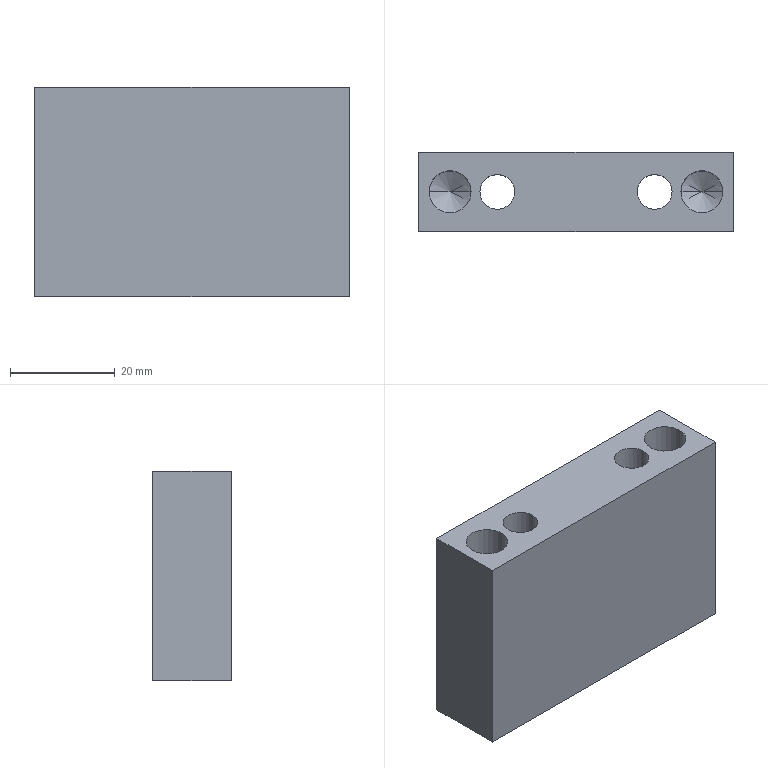Part | STEP file | 11-FG-SJ00611 | 1 solid | 24 faces | box 60 x 15 x 40 mm | volume 29373 mm3 | cylinder 12 | plane 8 | cone 4 | commonest cylinder face diameters 6.6 x4 8 x4 11 x4
STEP:
#1=CARTESIAN_POINT('',(-28.,0.,28.));
#2=VERTEX_POINT('',#1);
#3=CARTESIAN_POINT('',(-20.,0.,28.));
#4=VERTEX_POINT('',#3);
#5=CARTESIAN_POINT('',(-24.,0.,28.));
#6=DIRECTION('',(0.,0.,1.));
#7=DIRECTION('',(1.,0.,0.));
#8=AXIS2_PLACEMENT_3D('',#5,#6,#7);
#9=CIRCLE('',#8,4.);
#10=EDGE_CURVE('',#2,#4,#9,.T.);
#11=ORIENTED_EDGE('',*,*,#10,.F.);
#12=CARTESIAN_POINT('',(-28.,0.,40.));
#13=VERTEX_POINT('',#12);
#14=CARTESIAN_POINT('',(-28.,0.,40.));
#15=DIRECTION('',(0.,0.,1.));
#16=VECTOR('',#15,1000.);
#17=LINE('',#14,#16);
#18=EDGE_CURVE('',#2,#13,#17,.T.);
#19=ORIENTED_EDGE('',*,*,#18,.T.);
#20=CARTESIAN_POINT('',(-20.,0.,40.));
#21=VERTEX_POINT('',#20);
#22=CARTESIAN_POINT('',(-24.,0.,40.));
#23=DIRECTION('',(0.,0.,1.));
#24=DIRECTION('',(1.,0.,0.));
#25=AXIS2_PLACEMENT_3D('',#22,#23,#24);
#26=CIRCLE('',#25,4.);
#27=EDGE_CURVE('',#13,#21,#26,.T.);
#28=ORIENTED_EDGE('',*,*,#27,.T.);
#29=CARTESIAN_POINT('',(-20.,0.,40.));
#30=DIRECTION('',(0.,0.,1.));
#31=VECTOR('',#30,1000.);
#32=LINE('',#29,#31);
#33=EDGE_CURVE('',#4,#21,#32,.T.);
#34=ORIENTED_EDGE('',*,*,#33,.F.);
#35=EDGE_LOOP('',(#11,#19,#28,#34));
#36=FACE_OUTER_BOUND('',#35,.T.);
#37=CARTESIAN_POINT('',(-24.,0.,40.));
#38=DIRECTION('',(0.,0.,1.));
#39=DIRECTION('',(1.,0.,0.));
#40=AXIS2_PLACEMENT_3D('',#37,#38,#39);
#41=CYLINDRICAL_SURFACE('',#40,4.);
#42=ADVANCED_FACE('',(#36),#41,.F.);
#43=CARTESIAN_POINT('',(-24.,0.,25.597));
#44=VERTEX_POINT('',#43);
#45=CARTESIAN_POINT('',(-20.,0.,28.));
#46=DIRECTION('',(0.8572,0.,0.515));
#47=VECTOR('',#46,1000.);
#48=LINE('',#45,#47);
#49=EDGE_CURVE('',#44,#4,#48,.T.);
#50=ORIENTED_EDGE('',*,*,#49,.F.);
#51=CARTESIAN_POINT('',(-28.,0.,28.));
#52=DIRECTION('',(-0.8572,0.,0.515));
#53=VECTOR('',#52,1000.);
#54=LINE('',#51,#53);
#55=EDGE_CURVE('',#44,#2,#54,.T.);
#56=ORIENTED_EDGE('',*,*,#55,.T.);
#57=ORIENTED_EDGE('',*,*,#10,.T.);
#58=EDGE_LOOP('',(#50,#56,#57));
#59=FACE_OUTER_BOUND('',#58,.T.);
#60=CARTESIAN_POINT('',(-24.,0.,28.));
#61=DIRECTION('',(0.,0.,1.));
#62=DIRECTION('',(1.,0.,0.));
#63=AXIS2_PLACEMENT_3D('',#60,#61,#62);
#64=CONICAL_SURFACE('',#63,4.,1.03);
#65=ADVANCED_FACE('',(#59),#64,.F.);
#66=CARTESIAN_POINT('',(20.,0.,28.));
#67=VERTEX_POINT('',#66);
#68=CARTESIAN_POINT('',(28.,0.,28.));
#69=VERTEX_POINT('',#68);
#70=CARTESIAN_POINT('',(24.,0.,28.));
#71=DIRECTION('',(0.,0.,1.));
#72=DIRECTION('',(1.,0.,0.));
#73=AXIS2_PLACEMENT_3D('',#70,#71,#72);
#74=CIRCLE('',#73,4.);
#75=EDGE_CURVE('',#67,#69,#74,.T.);
#76=ORIENTED_EDGE('',*,*,#75,.F.);
#77=CARTESIAN_POINT('',(20.,0.,40.));
#78=VERTEX_POINT('',#77);
#79=CARTESIAN_POINT('',(20.,0.,40.));
#80=DIRECTION('',(0.,0.,1.));
#81=VECTOR('',#80,1000.);
#82=LINE('',#79,#81);
#83=EDGE_CURVE('',#67,#78,#82,.T.);
#84=ORIENTED_EDGE('',*,*,#83,.T.);
#85=CARTESIAN_POINT('',(28.,0.,40.));
#86=VERTEX_POINT('',#85);
#87=CARTESIAN_POINT('',(24.,0.,40.));
#88=DIRECTION('',(0.,0.,1.));
#89=DIRECTION('',(1.,0.,0.));
#90=AXIS2_PLACEMENT_3D('',#87,#88,#89);
#91=CIRCLE('',#90,4.);
#92=EDGE_CURVE('',#78,#86,#91,.T.);
#93=ORIENTED_EDGE('',*,*,#92,.T.);
#94=CARTESIAN_POINT('',(28.,0.,40.));
#95=DIRECTION('',(0.,0.,1.));
#96=VECTOR('',#95,1000.);
#97=LINE('',#94,#96);
#98=EDGE_CURVE('',#69,#86,#97,.T.);
#99=ORIENTED_EDGE('',*,*,#98,.F.);
#100=EDGE_LOOP('',(#76,#84,#93,#99));
#101=FACE_OUTER_BOUND('',#100,.T.);
#102=CARTESIAN_POINT('',(24.,0.,40.));
#103=DIRECTION('',(0.,0.,1.));
#104=DIRECTION('',(1.,0.,0.));
#105=AXIS2_PLACEMENT_3D('',#102,#103,#104);
#106=CYLINDRICAL_SURFACE('',#105,4.);
#107=ADVANCED_FACE('',(#101),#106,.F.);
#108=CARTESIAN_POINT('',(24.,0.,25.597));
#109=VERTEX_POINT('',#108);
#110=CARTESIAN_POINT('',(28.,0.,28.));
#111=DIRECTION('',(0.8572,0.,0.515));
#112=VECTOR('',#111,1000.);
#113=LINE('',#110,#112);
#114=EDGE_CURVE('',#109,#69,#113,.T.);
#115=ORIENTED_EDGE('',*,*,#114,.F.);
#116=CARTESIAN_POINT('',(20.,0.,28.));
#117=DIRECTION('',(-0.8572,0.,0.515));
#118=VECTOR('',#117,1000.);
#119=LINE('',#116,#118);
#120=EDGE_CURVE('',#109,#67,#119,.T.);
#121=ORIENTED_EDGE('',*,*,#120,.T.);
#122=ORIENTED_EDGE('',*,*,#75,.T.);
#123=EDGE_LOOP('',(#115,#121,#122));
#124=FACE_OUTER_BOUND('',#123,.T.);
#125=CARTESIAN_POINT('',(24.,0.,28.));
#126=DIRECTION('',(0.,0.,1.));
#127=DIRECTION('',(1.,0.,0.));
#128=AXIS2_PLACEMENT_3D('',#125,#126,#127);
#129=CONICAL_SURFACE('',#128,4.,1.03);
#130=ADVANCED_FACE('',(#124),#129,.F.);
#131=CARTESIAN_POINT('',(-9.5,0.,21.4));
#132=VERTEX_POINT('',#131);
#133=CARTESIAN_POINT('',(-20.5,0.,21.4));
#134=VERTEX_POINT('',#133);
#135=CARTESIAN_POINT('',(-15.,0.,21.4));
#136=DIRECTION('',(0.,0.,-1.));
#137=DIRECTION('',(-1.,0.,0.));
#138=AXIS2_PLACEMENT_3D('',#135,#136,#137);
#139=CIRCLE('',#138,5.5);
#140=EDGE_CURVE('',#132,#134,#139,.T.);
#141=ORIENTED_EDGE('',*,*,#140,.F.);
#142=CARTESIAN_POINT('',(-9.5,0.,0.));
#143=VERTEX_POINT('',#142);
#144=CARTESIAN_POINT('',(-9.5,0.,0.));
#145=DIRECTION('',(0.,0.,-1.));
#146=VECTOR('',#145,1000.);
#147=LINE('',#144,#146);
#148=EDGE_CURVE('',#132,#143,#147,.T.);
#149=ORIENTED_EDGE('',*,*,#148,.T.);
#150=CARTESIAN_POINT('',(-20.5,0.,0.));
#151=VERTEX_POINT('',#150);
#152=CARTESIAN_POINT('',(-15.,0.,0.));
#153=DIRECTION('',(0.,0.,-1.));
#154=DIRECTION('',(-1.,0.,0.));
#155=AXIS2_PLACEMENT_3D('',#152,#153,#154);
#156=CIRCLE('',#155,5.5);
#157=EDGE_CURVE('',#143,#151,#156,.T.);
#158=ORIENTED_EDGE('',*,*,#157,.T.);
#159=CARTESIAN_POINT('',(-20.5,0.,0.));
#160=DIRECTION('',(0.,0.,-1.));
#161=VECTOR('',#160,1000.);
#162=LINE('',#159,#161);
#163=EDGE_CURVE('',#134,#151,#162,.T.);
#164=ORIENTED_EDGE('',*,*,#163,.F.);
#165=EDGE_LOOP('',(#141,#149,#158,#164));
#166=FACE_OUTER_BOUND('',#165,.T.);
#167=CARTESIAN_POINT('',(-15.,0.,0.));
#168=DIRECTION('',(0.,0.,-1.));
#169=DIRECTION('',(-1.,0.,0.));
#170=AXIS2_PLACEMENT_3D('',#167,#168,#169);
#171=CYLINDRICAL_SURFACE('',#170,5.5);
#172=ADVANCED_FACE('',(#166),#171,.F.);
#173=CARTESIAN_POINT('',(-11.7,0.,40.));
#174=VERTEX_POINT('',#173);
#175=CARTESIAN_POINT('',(-18.3,0.,40.));
#176=VERTEX_POINT('',#175);
#177=CARTESIAN_POINT('',(-15.,0.,40.));
#178=DIRECTION('',(0.,0.,-1.));
#179=DIRECTION('',(-1.,0.,0.));
#180=AXIS2_PLACEMENT_3D('',#177,#178,#179);
#181=CIRCLE('',#180,3.3);
#182=EDGE_CURVE('',#174,#176,#181,.T.);
#183=ORIENTED_EDGE('',*,*,#182,.F.);
#184=CARTESIAN_POINT('',(-11.7,0.,21.4));
#185=VERTEX_POINT('',#184);
#186=CARTESIAN_POINT('',(-11.7,0.,0.));
#187=DIRECTION('',(0.,0.,-1.));
#188=VECTOR('',#187,1000.);
#189=LINE('',#186,#188);
#190=EDGE_CURVE('',#174,#185,#189,.T.);
#191=ORIENTED_EDGE('',*,*,#190,.T.);
#192=CARTESIAN_POINT('',(-18.3,0.,21.4));
#193=VERTEX_POINT('',#192);
#194=CARTESIAN_POINT('',(-15.,0.,21.4));
#195=DIRECTION('',(0.,0.,-1.));
#196=DIRECTION('',(-1.,0.,0.));
#197=AXIS2_PLACEMENT_3D('',#194,#195,#196);
#198=CIRCLE('',#197,3.3);
#199=EDGE_CURVE('',#185,#193,#198,.T.);
#200=ORIENTED_EDGE('',*,*,#199,.T.);
#201=CARTESIAN_POINT('',(-18.3,0.,0.));
#202=DIRECTION('',(0.,0.,-1.));
#203=VECTOR('',#202,1000.);
#204=LINE('',#201,#203);
#205=EDGE_CURVE('',#176,#193,#204,.T.);
#206=ORIENTED_EDGE('',*,*,#205,.F.);
#207=EDGE_LOOP('',(#183,#191,#200,#206));
#208=FACE_OUTER_BOUND('',#207,.T.);
#209=CARTESIAN_POINT('',(-15.,0.,0.));
#210=DIRECTION('',(0.,0.,-1.));
#211=DIRECTION('',(-1.,0.,0.));
#212=AXIS2_PLACEMENT_3D('',#209,#210,#211);
#213=CYLINDRICAL_SURFACE('',#212,3.3);
#214=ADVANCED_FACE('',(#208),#213,.F.);
#215=CARTESIAN_POINT('',(20.5,0.,21.4));
#216=VERTEX_POINT('',#215);
#217=CARTESIAN_POINT('',(9.5,0.,21.4));
#218=VERTEX_POINT('',#217);
#219=CARTESIAN_POINT('',(15.,0.,21.4));
#220=DIRECTION('',(0.,0.,-1.));
#221=DIRECTION('',(-1.,0.,0.));
#222=AXIS2_PLACEMENT_3D('',#219,#220,#221);
#223=CIRCLE('',#222,5.5);
#224=EDGE_CURVE('',#216,#218,#223,.T.);
#225=ORIENTED_EDGE('',*,*,#224,.F.);
#226=CARTESIAN_POINT('',(20.5,0.,0.));
#227=VERTEX_POINT('',#226);
#228=CARTESIAN_POINT('',(20.5,0.,0.));
#229=DIRECTION('',(0.,0.,-1.));
#230=VECTOR('',#229,1000.);
#231=LINE('',#228,#230);
#232=EDGE_CURVE('',#216,#227,#231,.T.);
#233=ORIENTED_EDGE('',*,*,#232,.T.);
#234=CARTESIAN_POINT('',(9.5,0.,0.));
#235=VERTEX_POINT('',#234);
#236=CARTESIAN_POINT('',(15.,0.,0.));
#237=DIRECTION('',(0.,0.,-1.));
#238=DIRECTION('',(-1.,0.,0.));
#239=AXIS2_PLACEMENT_3D('',#236,#237,#238);
#240=CIRCLE('',#239,5.5);
#241=EDGE_CURVE('',#227,#235,#240,.T.);
#242=ORIENTED_EDGE('',*,*,#241,.T.);
#243=CARTESIAN_POINT('',(9.5,0.,0.));
#244=DIRECTION('',(0.,0.,-1.));
#245=VECTOR('',#244,1000.);
#246=LINE('',#243,#245);
#247=EDGE_CURVE('',#218,#235,#246,.T.);
#248=ORIENTED_EDGE('',*,*,#247,.F.);
#249=EDGE_LOOP('',(#225,#233,#242,#248));
#250=FACE_OUTER_BOUND('',#249,.T.);
#251=CARTESIAN_POINT('',(15.,0.,0.));
#252=DIRECTION('',(0.,0.,-1.));
#253=DIRECTION('',(-1.,0.,0.));
#254=AXIS2_PLACEMENT_3D('',#251,#252,#253);
#255=CYLINDRICAL_SURFACE('',#254,5.5);
#256=ADVANCED_FACE('',(#250),#255,.F.);
#257=CARTESIAN_POINT('',(18.3,0.,40.));
#258=VERTEX_POINT('',#257);
#259=CARTESIAN_POINT('',(11.7,0.,40.));
#260=VERTEX_POINT('',#259);
#261=CARTESIAN_POINT('',(15.,0.,40.));
#262=DIRECTION('',(0.,0.,-1.));
#263=DIRECTION('',(-1.,0.,0.));
#264=AXIS2_PLACEMENT_3D('',#261,#262,#263);
#265=CIRCLE('',#264,3.3);
#266=EDGE_CURVE('',#258,#260,#265,.T.);
#267=ORIENTED_EDGE('',*,*,#266,.F.);
#268=CARTESIAN_POINT('',(18.3,0.,21.4));
#269=VERTEX_POINT('',#268);
#270=CARTESIAN_POINT('',(18.3,0.,0.));
#271=DIRECTION('',(0.,0.,-1.));
#272=VECTOR('',#271,1000.);
#273=LINE('',#270,#272);
#274=EDGE_CURVE('',#258,#269,#273,.T.);
#275=ORIENTED_EDGE('',*,*,#274,.T.);
#276=CARTESIAN_POINT('',(11.7,0.,21.4));
#277=VERTEX_POINT('',#276);
#278=CARTESIAN_POINT('',(15.,0.,21.4));
#279=DIRECTION('',(0.,0.,-1.));
#280=DIRECTION('',(-1.,0.,0.));
#281=AXIS2_PLACEMENT_3D('',#278,#279,#280);
#282=CIRCLE('',#281,3.3);
#283=EDGE_CURVE('',#269,#277,#282,.T.);
#284=ORIENTED_EDGE('',*,*,#283,.T.);
#285=CARTESIAN_POINT('',(11.7,0.,0.));
#286=DIRECTION('',(0.,0.,-1.));
#287=VECTOR('',#286,1000.);
#288=LINE('',#285,#287);
#289=EDGE_CURVE('',#260,#277,#288,.T.);
#290=ORIENTED_EDGE('',*,*,#289,.F.);
#291=EDGE_LOOP('',(#267,#275,#284,#290));
#292=FACE_OUTER_BOUND('',#291,.T.);
#293=CARTESIAN_POINT('',(15.,0.,0.));
#294=DIRECTION('',(0.,0.,-1.));
#295=DIRECTION('',(-1.,0.,0.));
#296=AXIS2_PLACEMENT_3D('',#293,#294,#295);
#297=CYLINDRICAL_SURFACE('',#296,3.3);
#298=ADVANCED_FACE('',(#292),#297,.F.);
#299=CARTESIAN_POINT('',(-30.,7.5,0.));
#300=VERTEX_POINT('',#299);
#301=CARTESIAN_POINT('',(-30.,-7.5,0.));
#302=VERTEX_POINT('',#301);
#303=CARTESIAN_POINT('',(-30.,-7.5,0.));
#304=DIRECTION('',(0.,-1.,0.));
#305=VECTOR('',#304,1000.);
#306=LINE('',#303,#305);
#307=EDGE_CURVE('',#300,#302,#306,.T.);
#308=ORIENTED_EDGE('',*,*,#307,.T.);
#309=CARTESIAN_POINT('',(-30.,-7.5,40.));
#310=VERTEX_POINT('',#309);
#311=CARTESIAN_POINT('',(-30.,-7.5,40.));
#312=DIRECTION('',(0.,0.,-1.));
#313=VECTOR('',#312,1000.);
#314=LINE('',#311,#313);
#315=EDGE_CURVE('',#310,#302,#314,.T.);
#316=ORIENTED_EDGE('',*,*,#315,.F.);
#317=CARTESIAN_POINT('',(-30.,7.5,40.));
#318=VERTEX_POINT('',#317);
#319=CARTESIAN_POINT('',(-30.,-7.5,40.));
#320=DIRECTION('',(0.,-1.,0.));
#321=VECTOR('',#320,1000.);
#322=LINE('',#319,#321);
#323=EDGE_CURVE('',#318,#310,#322,.T.);
#324=ORIENTED_EDGE('',*,*,#323,.F.);
#325=CARTESIAN_POINT('',(-30.,7.5,40.));
#326=DIRECTION('',(0.,0.,-1.));
#327=VECTOR('',#326,1000.);
#328=LINE('',#325,#327);
#329=EDGE_CURVE('',#318,#300,#328,.T.);
#330=ORIENTED_EDGE('',*,*,#329,.T.);
#331=EDGE_LOOP('',(#308,#316,#324,#330));
#332=FACE_OUTER_BOUND('',#331,.T.);
#333=CARTESIAN_POINT('',(-30.,-7.5,40.));
#334=DIRECTION('',(1.,0.,0.));
#335=DIRECTION('',(0.,0.,-1.));
#336=AXIS2_PLACEMENT_3D('',#333,#334,#335);
#337=PLANE('',#336);
#338=ADVANCED_FACE('',(#332),#337,.F.);
#339=CARTESIAN_POINT('',(30.,-7.5,0.));
#340=VERTEX_POINT('',#339);
#341=CARTESIAN_POINT('',(30.,-7.5,0.));
#342=DIRECTION('',(1.,0.,0.));
#343=VECTOR('',#342,1000.);
#344=LINE('',#341,#343);
#345=EDGE_CURVE('',#302,#340,#344,.T.);
#346=ORIENTED_EDGE('',*,*,#345,.T.);
#347=CARTESIAN_POINT('',(30.,-7.5,40.));
#348=VERTEX_POINT('',#347);
#349=CARTESIAN_POINT('',(30.,-7.5,40.));
#350=DIRECTION('',(0.,0.,-1.));
#351=VECTOR('',#350,1000.);
#352=LINE('',#349,#351);
#353=EDGE_CURVE('',#348,#340,#352,.T.);
#354=ORIENTED_EDGE('',*,*,#353,.F.);
#355=CARTESIAN_POINT('',(30.,-7.5,40.));
#356=DIRECTION('',(1.,0.,0.));
#357=VECTOR('',#356,1000.);
#358=LINE('',#355,#357);
#359=EDGE_CURVE('',#310,#348,#358,.T.);
#360=ORIENTED_EDGE('',*,*,#359,.F.);
#361=ORIENTED_EDGE('',*,*,#315,.T.);
#362=EDGE_LOOP('',(#346,#354,#360,#361));
#363=FACE_OUTER_BOUND('',#362,.T.);
#364=CARTESIAN_POINT('',(30.,-7.5,40.));
#365=DIRECTION('',(0.,1.,0.));
#366=DIRECTION('',(-1.,0.,0.));
#367=AXIS2_PLACEMENT_3D('',#364,#365,#366);
#368=PLANE('',#367);
#369=ADVANCED_FACE('',(#363),#368,.F.);
#370=CARTESIAN_POINT('',(30.,7.5,0.));
#371=VERTEX_POINT('',#370);
#372=CARTESIAN_POINT('',(30.,-7.5,0.));
#373=DIRECTION('',(0.,1.,0.));
#374=VECTOR('',#373,1000.);
#375=LINE('',#372,#374);
#376=EDGE_CURVE('',#340,#371,#375,.T.);
#377=ORIENTED_EDGE('',*,*,#376,.T.);
#378=CARTESIAN_POINT('',(30.,7.5,40.));
#379=VERTEX_POINT('',#378);
#380=CARTESIAN_POINT('',(30.,7.5,40.));
#381=DIRECTION('',(0.,0.,-1.));
#382=VECTOR('',#381,1000.);
#383=LINE('',#380,#382);
#384=EDGE_CURVE('',#379,#371,#383,.T.);
#385=ORIENTED_EDGE('',*,*,#384,.F.);
#386=CARTESIAN_POINT('',(30.,-7.5,40.));
#387=DIRECTION('',(0.,1.,0.));
#388=VECTOR('',#387,1000.);
#389=LINE('',#386,#388);
#390=EDGE_CURVE('',#348,#379,#389,.T.);
#391=ORIENTED_EDGE('',*,*,#390,.F.);
#392=ORIENTED_EDGE('',*,*,#353,.T.);
#393=EDGE_LOOP('',(#377,#385,#391,#392));
#394=FACE_OUTER_BOUND('',#393,.T.);
#395=CARTESIAN_POINT('',(30.,-7.5,40.));
#396=DIRECTION('',(-1.,0.,0.));
#397=DIRECTION('',(0.,0.,1.));
#398=AXIS2_PLACEMENT_3D('',#395,#396,#397);
#399=PLANE('',#398);
#400=ADVANCED_FACE('',(#394),#399,.F.);
#401=CARTESIAN_POINT('',(30.,7.5,0.));
#402=DIRECTION('',(-1.,0.,0.));
#403=VECTOR('',#402,1000.);
#404=LINE('',#401,#403);
#405=EDGE_CURVE('',#371,#300,#404,.T.);
#406=ORIENTED_EDGE('',*,*,#405,.T.);
#407=ORIENTED_EDGE('',*,*,#329,.F.);
#408=CARTESIAN_POINT('',(30.,7.5,40.));
#409=DIRECTION('',(-1.,0.,0.));
#410=VECTOR('',#409,1000.);
#411=LINE('',#408,#410);
#412=EDGE_CURVE('',#379,#318,#411,.T.);
#413=ORIENTED_EDGE('',*,*,#412,.F.);
#414=ORIENTED_EDGE('',*,*,#384,.T.);
#415=EDGE_LOOP('',(#406,#407,#413,#414));
#416=FACE_OUTER_BOUND('',#415,.T.);
#417=CARTESIAN_POINT('',(30.,7.5,40.));
#418=DIRECTION('',(0.,-1.,0.));
#419=DIRECTION('',(1.,0.,0.));
#420=AXIS2_PLACEMENT_3D('',#417,#418,#419);
#421=PLANE('',#420);
#422=ADVANCED_FACE('',(#416),#421,.F.);
#423=CARTESIAN_POINT('',(-24.,0.,40.));
#424=DIRECTION('',(0.,0.,1.));
#425=DIRECTION('',(1.,0.,0.));
#426=AXIS2_PLACEMENT_3D('',#423,#424,#425);
#427=CIRCLE('',#426,4.);
#428=EDGE_CURVE('',#21,#13,#427,.T.);
#429=ORIENTED_EDGE('',*,*,#428,.F.);
#430=ORIENTED_EDGE('',*,*,#27,.F.);
#431=EDGE_LOOP('',(#429,#430));
#432=FACE_BOUND('',#431,.T.);
#433=CARTESIAN_POINT('',(24.,0.,40.));
#434=DIRECTION('',(0.,0.,1.));
#435=DIRECTION('',(1.,0.,0.));
#436=AXIS2_PLACEMENT_3D('',#433,#434,#435);
#437=CIRCLE('',#436,4.);
#438=EDGE_CURVE('',#86,#78,#437,.T.);
#439=ORIENTED_EDGE('',*,*,#438,.F.);
#440=ORIENTED_EDGE('',*,*,#92,.F.);
#441=EDGE_LOOP('',(#439,#440));
#442=FACE_BOUND('',#441,.T.);
#443=CARTESIAN_POINT('',(-15.,0.,40.));
#444=DIRECTION('',(0.,0.,-1.));
#445=DIRECTION('',(-1.,0.,0.));
#446=AXIS2_PLACEMENT_3D('',#443,#444,#445);
#447=CIRCLE('',#446,3.3);
#448=EDGE_CURVE('',#176,#174,#447,.T.);
#449=ORIENTED_EDGE('',*,*,#448,.T.);
#450=ORIENTED_EDGE('',*,*,#182,.T.);
#451=EDGE_LOOP('',(#449,#450));
#452=FACE_BOUND('',#451,.T.);
#453=CARTESIAN_POINT('',(15.,0.,40.));
#454=DIRECTION('',(0.,0.,-1.));
#455=DIRECTION('',(-1.,0.,0.));
#456=AXIS2_PLACEMENT_3D('',#453,#454,#455);
#457=CIRCLE('',#456,3.3);
#458=EDGE_CURVE('',#260,#258,#457,.T.);
#459=ORIENTED_EDGE('',*,*,#458,.T.);
#460=ORIENTED_EDGE('',*,*,#266,.T.);
#461=EDGE_LOOP('',(#459,#460));
#462=FACE_BOUND('',#461,.T.);
#463=ORIENTED_EDGE('',*,*,#323,.T.);
#464=ORIENTED_EDGE('',*,*,#359,.T.);
#465=ORIENTED_EDGE('',*,*,#390,.T.);
#466=ORIENTED_EDGE('',*,*,#412,.T.);
#467=EDGE_LOOP('',(#463,#464,#465,#466));
#468=FACE_OUTER_BOUND('',#467,.T.);
#469=CARTESIAN_POINT('',(0.,0.,40.));
#470=DIRECTION('',(0.,0.,1.));
#471=DIRECTION('',(1.,0.,0.));
#472=AXIS2_PLACEMENT_3D('',#469,#470,#471);
#473=PLANE('',#472);
#474=ADVANCED_FACE('',(#432,#442,#452,#462,#468),#473,.T.);
#475=CARTESIAN_POINT('',(-15.,0.,0.));
#476=DIRECTION('',(0.,0.,-1.));
#477=DIRECTION('',(-1.,0.,0.));
#478=AXIS2_PLACEMENT_3D('',#475,#476,#477);
#479=CIRCLE('',#478,5.5);
#480=EDGE_CURVE('',#151,#143,#479,.T.);
#481=ORIENTED_EDGE('',*,*,#480,.F.);
#482=ORIENTED_EDGE('',*,*,#157,.F.);
#483=EDGE_LOOP('',(#481,#482));
#484=FACE_BOUND('',#483,.T.);
#485=CARTESIAN_POINT('',(15.,0.,0.));
#486=DIRECTION('',(0.,0.,-1.));
#487=DIRECTION('',(-1.,0.,0.));
#488=AXIS2_PLACEMENT_3D('',#485,#486,#487);
#489=CIRCLE('',#488,5.5);
#490=EDGE_CURVE('',#235,#227,#489,.T.);
#491=ORIENTED_EDGE('',*,*,#490,.F.);
#492=ORIENTED_EDGE('',*,*,#241,.F.);
#493=EDGE_LOOP('',(#491,#492));
#494=FACE_BOUND('',#493,.T.);
#495=ORIENTED_EDGE('',*,*,#307,.F.);
#496=ORIENTED_EDGE('',*,*,#405,.F.);
#497=ORIENTED_EDGE('',*,*,#376,.F.);
#498=ORIENTED_EDGE('',*,*,#345,.F.);
#499=EDGE_LOOP('',(#495,#496,#497,#498));
#500=FACE_OUTER_BOUND('',#499,.T.);
#501=CARTESIAN_POINT('',(0.,0.,0.));
#502=DIRECTION('',(0.,0.,1.));
#503=DIRECTION('',(1.,0.,0.));
#504=AXIS2_PLACEMENT_3D('',#501,#502,#503);
#505=PLANE('',#504);
#506=ADVANCED_FACE('',(#484,#494,#500),#505,.F.);
#507=ORIENTED_EDGE('',*,*,#274,.F.);
#508=ORIENTED_EDGE('',*,*,#458,.F.);
#509=ORIENTED_EDGE('',*,*,#289,.T.);
#510=CARTESIAN_POINT('',(15.,0.,21.4));
#511=DIRECTION('',(0.,0.,-1.));
#512=DIRECTION('',(-1.,0.,0.));
#513=AXIS2_PLACEMENT_3D('',#510,#511,#512);
#514=CIRCLE('',#513,3.3);
#515=EDGE_CURVE('',#277,#269,#514,.T.);
#516=ORIENTED_EDGE('',*,*,#515,.T.);
#517=EDGE_LOOP('',(#507,#508,#509,#516));
#518=FACE_OUTER_BOUND('',#517,.T.);
#519=CARTESIAN_POINT('',(15.,0.,0.));
#520=DIRECTION('',(0.,0.,-1.));
#521=DIRECTION('',(-1.,0.,0.));
#522=AXIS2_PLACEMENT_3D('',#519,#520,#521);
#523=CYLINDRICAL_SURFACE('',#522,3.3);
#524=ADVANCED_FACE('',(#518),#523,.F.);
#525=ORIENTED_EDGE('',*,*,#515,.F.);
#526=ORIENTED_EDGE('',*,*,#283,.F.);
#527=EDGE_LOOP('',(#525,#526));
#528=FACE_BOUND('',#527,.T.);
#529=CARTESIAN_POINT('',(15.,0.,21.4));
#530=DIRECTION('',(0.,0.,-1.));
#531=DIRECTION('',(-1.,0.,0.));
#532=AXIS2_PLACEMENT_3D('',#529,#530,#531);
#533=CIRCLE('',#532,5.5);
#534=EDGE_CURVE('',#218,#216,#533,.T.);
#535=ORIENTED_EDGE('',*,*,#534,.T.);
#536=ORIENTED_EDGE('',*,*,#224,.T.);
#537=EDGE_LOOP('',(#535,#536));
#538=FACE_OUTER_BOUND('',#537,.T.);
#539=CARTESIAN_POINT('',(18.3,0.,21.4));
#540=DIRECTION('',(0.,0.,1.));
#541=DIRECTION('',(1.,0.,0.));
#542=AXIS2_PLACEMENT_3D('',#539,#540,#541);
#543=PLANE('',#542);
#544=ADVANCED_FACE('',(#528,#538),#543,.F.);
#545=ORIENTED_EDGE('',*,*,#232,.F.);
#546=ORIENTED_EDGE('',*,*,#534,.F.);
#547=ORIENTED_EDGE('',*,*,#247,.T.);
#548=ORIENTED_EDGE('',*,*,#490,.T.);
#549=EDGE_LOOP('',(#545,#546,#547,#548));
#550=FACE_OUTER_BOUND('',#549,.T.);
#551=CARTESIAN_POINT('',(15.,0.,0.));
#552=DIRECTION('',(0.,0.,-1.));
#553=DIRECTION('',(-1.,0.,0.));
#554=AXIS2_PLACEMENT_3D('',#551,#552,#553);
#555=CYLINDRICAL_SURFACE('',#554,5.5);
#556=ADVANCED_FACE('',(#550),#555,.F.);
#557=ORIENTED_EDGE('',*,*,#190,.F.);
#558=ORIENTED_EDGE('',*,*,#448,.F.);
#559=ORIENTED_EDGE('',*,*,#205,.T.);
#560=CARTESIAN_POINT('',(-15.,0.,21.4));
#561=DIRECTION('',(0.,0.,-1.));
#562=DIRECTION('',(-1.,0.,0.));
#563=AXIS2_PLACEMENT_3D('',#560,#561,#562);
#564=CIRCLE('',#563,3.3);
#565=EDGE_CURVE('',#193,#185,#564,.T.);
#566=ORIENTED_EDGE('',*,*,#565,.T.);
#567=EDGE_LOOP('',(#557,#558,#559,#566));
#568=FACE_OUTER_BOUND('',#567,.T.);
#569=CARTESIAN_POINT('',(-15.,0.,0.));
#570=DIRECTION('',(0.,0.,-1.));
#571=DIRECTION('',(-1.,0.,0.));
#572=AXIS2_PLACEMENT_3D('',#569,#570,#571);
#573=CYLINDRICAL_SURFACE('',#572,3.3);
#574=ADVANCED_FACE('',(#568),#573,.F.);
#575=ORIENTED_EDGE('',*,*,#565,.F.);
#576=ORIENTED_EDGE('',*,*,#199,.F.);
#577=EDGE_LOOP('',(#575,#576));
#578=FACE_BOUND('',#577,.T.);
#579=CARTESIAN_POINT('',(-15.,0.,21.4));
#580=DIRECTION('',(0.,0.,-1.));
#581=DIRECTION('',(-1.,0.,0.));
#582=AXIS2_PLACEMENT_3D('',#579,#580,#581);
#583=CIRCLE('',#582,5.5);
#584=EDGE_CURVE('',#134,#132,#583,.T.);
#585=ORIENTED_EDGE('',*,*,#584,.T.);
#586=ORIENTED_EDGE('',*,*,#140,.T.);
#587=EDGE_LOOP('',(#585,#586));
#588=FACE_OUTER_BOUND('',#587,.T.);
#589=CARTESIAN_POINT('',(-11.7,0.,21.4));
#590=DIRECTION('',(0.,0.,1.));
#591=DIRECTION('',(1.,0.,0.));
#592=AXIS2_PLACEMENT_3D('',#589,#590,#591);
#593=PLANE('',#592);
#594=ADVANCED_FACE('',(#578,#588),#593,.F.);
#595=ORIENTED_EDGE('',*,*,#148,.F.);
#596=ORIENTED_EDGE('',*,*,#584,.F.);
#597=ORIENTED_EDGE('',*,*,#163,.T.);
#598=ORIENTED_EDGE('',*,*,#480,.T.);
#599=EDGE_LOOP('',(#595,#596,#597,#598));
#600=FACE_OUTER_BOUND('',#599,.T.);
#601=CARTESIAN_POINT('',(-15.,0.,0.));
#602=DIRECTION('',(0.,0.,-1.));
#603=DIRECTION('',(-1.,0.,0.));
#604=AXIS2_PLACEMENT_3D('',#601,#602,#603);
#605=CYLINDRICAL_SURFACE('',#604,5.5);
#606=ADVANCED_FACE('',(#600),#605,.F.);
#607=ORIENTED_EDGE('',*,*,#120,.F.);
#608=ORIENTED_EDGE('',*,*,#114,.T.);
#609=CARTESIAN_POINT('',(24.,0.,28.));
#610=DIRECTION('',(0.,0.,1.));
#611=DIRECTION('',(1.,0.,0.));
#612=AXIS2_PLACEMENT_3D('',#609,#610,#611);
#613=CIRCLE('',#612,4.);
#614=EDGE_CURVE('',#69,#67,#613,.T.);
#615=ORIENTED_EDGE('',*,*,#614,.T.);
#616=EDGE_LOOP('',(#607,#608,#615));
#617=FACE_OUTER_BOUND('',#616,.T.);
#618=CARTESIAN_POINT('',(24.,0.,28.));
#619=DIRECTION('',(0.,0.,1.));
#620=DIRECTION('',(1.,0.,0.));
#621=AXIS2_PLACEMENT_3D('',#618,#619,#620);
#622=CONICAL_SURFACE('',#621,4.,1.03);
#623=ADVANCED_FACE('',(#617),#622,.F.);
#624=ORIENTED_EDGE('',*,*,#83,.F.);
#625=ORIENTED_EDGE('',*,*,#614,.F.);
#626=ORIENTED_EDGE('',*,*,#98,.T.);
#627=ORIENTED_EDGE('',*,*,#438,.T.);
#628=EDGE_LOOP('',(#624,#625,#626,#627));
#629=FACE_OUTER_BOUND('',#628,.T.);
#630=CARTESIAN_POINT('',(24.,0.,40.));
#631=DIRECTION('',(0.,0.,1.));
#632=DIRECTION('',(1.,0.,0.));
#633=AXIS2_PLACEMENT_3D('',#630,#631,#632);
#634=CYLINDRICAL_SURFACE('',#633,4.);
#635=ADVANCED_FACE('',(#629),#634,.F.);
#636=ORIENTED_EDGE('',*,*,#55,.F.);
#637=ORIENTED_EDGE('',*,*,#49,.T.);
#638=CARTESIAN_POINT('',(-24.,0.,28.));
#639=DIRECTION('',(0.,0.,1.));
#640=DIRECTION('',(1.,0.,0.));
#641=AXIS2_PLACEMENT_3D('',#638,#639,#640);
#642=CIRCLE('',#641,4.);
#643=EDGE_CURVE('',#4,#2,#642,.T.);
#644=ORIENTED_EDGE('',*,*,#643,.T.);
#645=EDGE_LOOP('',(#636,#637,#644));
#646=FACE_OUTER_BOUND('',#645,.T.);
#647=CARTESIAN_POINT('',(-24.,0.,28.));
#648=DIRECTION('',(0.,0.,1.));
#649=DIRECTION('',(1.,0.,0.));
#650=AXIS2_PLACEMENT_3D('',#647,#648,#649);
#651=CONICAL_SURFACE('',#650,4.,1.03);
#652=ADVANCED_FACE('',(#646),#651,.F.);
#653=ORIENTED_EDGE('',*,*,#18,.F.);
#654=ORIENTED_EDGE('',*,*,#643,.F.);
#655=ORIENTED_EDGE('',*,*,#33,.T.);
#656=ORIENTED_EDGE('',*,*,#428,.T.);
#657=EDGE_LOOP('',(#653,#654,#655,#656));
#658=FACE_OUTER_BOUND('',#657,.T.);
#659=CARTESIAN_POINT('',(-24.,0.,40.));
#660=DIRECTION('',(0.,0.,1.));
#661=DIRECTION('',(1.,0.,0.));
#662=AXIS2_PLACEMENT_3D('',#659,#660,#661);
#663=CYLINDRICAL_SURFACE('',#662,4.);
#664=ADVANCED_FACE('',(#658),#663,.F.);
#665=CLOSED_SHELL('',(#42,#65,#107,#130,#172,#214,#256,#298,#338,#369,#400,#422,#474,#506,#524,#544,#556,#574,#594,#606,#623,#635,#652,#664));
#666=MANIFOLD_SOLID_BREP('',#665);
#667=CARTESIAN_POINT('',(0.,0.,0.));
#668=DIRECTION('',(0.,0.,1.));
#669=DIRECTION('',(1.,0.,0.));
#670=AXIS2_PLACEMENT_3D('',#667,#668,#669);
#671=(LENGTH_UNIT()NAMED_UNIT(*)SI_UNIT(.MILLI.,.METRE.));
#672=UNCERTAINTY_MEASURE_WITH_UNIT(LENGTH_MEASURE(0.00001),#671,'','');
#673=(NAMED_UNIT(*)PLANE_ANGLE_UNIT()SI_UNIT($,.RADIAN.));
#674=(NAMED_UNIT(*)SI_UNIT($,.STERADIAN.)SOLID_ANGLE_UNIT());
#675=(GEOMETRIC_REPRESENTATION_CONTEXT(3)GLOBAL_UNCERTAINTY_ASSIGNED_CONTEXT((#672))GLOBAL_UNIT_ASSIGNED_CONTEXT((#671,#673,#674))REPRESENTATION_CONTEXT('',''));
#676=ADVANCED_BREP_SHAPE_REPRESENTATION('',(#666,#670),#675);